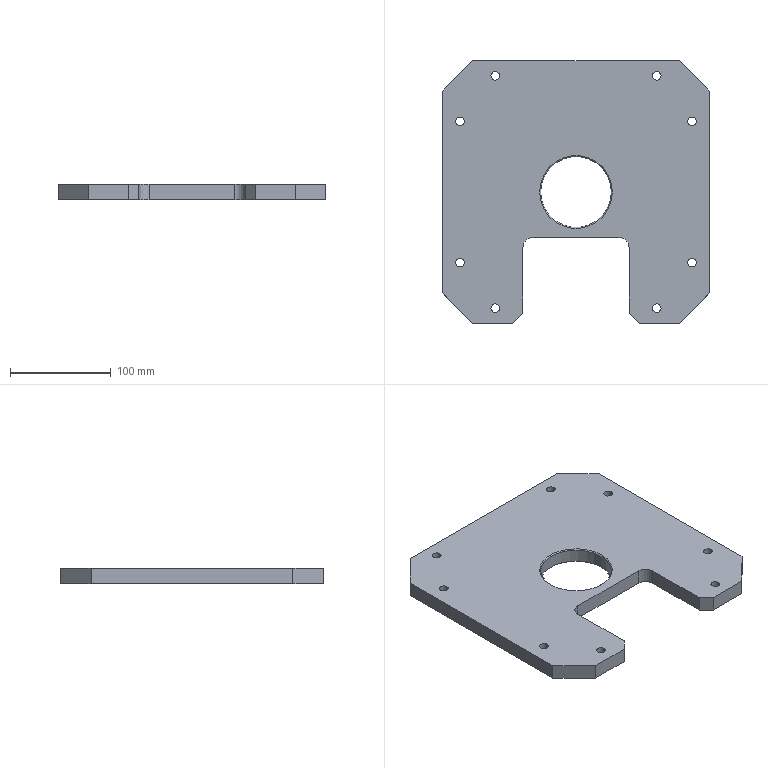Part | SolidWorks | features Chamfer 3, Cut 1, Extrusion 1, Fillet 1, HoleWzd 1, ICE 1 | 1 solid | 40 faces | box 265 x 260 x 15 mm | volume 807011 mm3 | cylinder 20 | plane 16 | cone 4 | commonest cylinder face diameters 8.5 x16 20 x2 70 x2
STEP:
#1=CARTESIAN_POINT('',(-35.,0.,14.));
#2=VERTEX_POINT('',#1);
#3=CARTESIAN_POINT('',(35.,0.,14.));
#4=VERTEX_POINT('',#3);
#5=CARTESIAN_POINT('',(0.,0.,14.));
#6=DIRECTION('',(0.,0.,1.));
#7=DIRECTION('',(-1.,0.,0.));
#8=AXIS2_PLACEMENT_3D('',#5,#6,#7);
#9=CIRCLE('',#8,35.);
#10=EDGE_CURVE('',#2,#4,#9,.T.);
#11=ORIENTED_EDGE('',*,*,#10,.F.);
#12=CARTESIAN_POINT('',(-36.,0.,15.));
#13=VERTEX_POINT('',#12);
#14=CARTESIAN_POINT('',(-36.,0.,15.));
#15=DIRECTION('',(-0.7071,0.,0.7071));
#16=VECTOR('',#15,1000.);
#17=LINE('',#14,#16);
#18=EDGE_CURVE('',#2,#13,#17,.T.);
#19=ORIENTED_EDGE('',*,*,#18,.T.);
#20=CARTESIAN_POINT('',(36.,0.,15.));
#21=VERTEX_POINT('',#20);
#22=CARTESIAN_POINT('',(0.,0.,15.));
#23=DIRECTION('',(0.,0.,-1.));
#24=DIRECTION('',(-1.,0.,0.));
#25=AXIS2_PLACEMENT_3D('',#22,#23,#24);
#26=CIRCLE('',#25,36.);
#27=EDGE_CURVE('',#21,#13,#26,.T.);
#28=ORIENTED_EDGE('',*,*,#27,.F.);
#29=CARTESIAN_POINT('',(36.,0.,15.));
#30=DIRECTION('',(0.7071,0.,0.7071));
#31=VECTOR('',#30,1000.);
#32=LINE('',#29,#31);
#33=EDGE_CURVE('',#4,#21,#32,.T.);
#34=ORIENTED_EDGE('',*,*,#33,.F.);
#35=EDGE_LOOP('',(#11,#19,#28,#34));
#36=FACE_OUTER_BOUND('',#35,.T.);
#37=CARTESIAN_POINT('',(0.,0.,15.));
#38=DIRECTION('',(0.,0.,1.));
#39=DIRECTION('',(1.,0.,0.));
#40=AXIS2_PLACEMENT_3D('',#37,#38,#39);
#41=CONICAL_SURFACE('',#40,36.,0.7854);
#42=ADVANCED_FACE('',(#36),#41,.F.);
#43=CARTESIAN_POINT('',(35.,0.,1.));
#44=VERTEX_POINT('',#43);
#45=CARTESIAN_POINT('',(-35.,0.,1.));
#46=VERTEX_POINT('',#45);
#47=CARTESIAN_POINT('',(0.,0.,1.));
#48=DIRECTION('',(0.,0.,-1.));
#49=DIRECTION('',(-1.,0.,0.));
#50=AXIS2_PLACEMENT_3D('',#47,#48,#49);
#51=CIRCLE('',#50,35.);
#52=EDGE_CURVE('',#44,#46,#51,.T.);
#53=ORIENTED_EDGE('',*,*,#52,.F.);
#54=CARTESIAN_POINT('',(36.,0.,0.));
#55=VERTEX_POINT('',#54);
#56=CARTESIAN_POINT('',(35.,0.,1.));
#57=DIRECTION('',(0.7071,0.,-0.7071));
#58=VECTOR('',#57,1000.);
#59=LINE('',#56,#58);
#60=EDGE_CURVE('',#44,#55,#59,.T.);
#61=ORIENTED_EDGE('',*,*,#60,.T.);
#62=CARTESIAN_POINT('',(-36.,0.,0.));
#63=VERTEX_POINT('',#62);
#64=CARTESIAN_POINT('',(0.,0.,0.));
#65=DIRECTION('',(0.,0.,1.));
#66=DIRECTION('',(-1.,0.,0.));
#67=AXIS2_PLACEMENT_3D('',#64,#65,#66);
#68=CIRCLE('',#67,36.);
#69=EDGE_CURVE('',#63,#55,#68,.T.);
#70=ORIENTED_EDGE('',*,*,#69,.F.);
#71=CARTESIAN_POINT('',(-35.,0.,1.));
#72=DIRECTION('',(-0.7071,0.,-0.7071));
#73=VECTOR('',#72,1000.);
#74=LINE('',#71,#73);
#75=EDGE_CURVE('',#46,#63,#74,.T.);
#76=ORIENTED_EDGE('',*,*,#75,.F.);
#77=EDGE_LOOP('',(#53,#61,#70,#76));
#78=FACE_OUTER_BOUND('',#77,.T.);
#79=CARTESIAN_POINT('',(0.,0.,1.));
#80=DIRECTION('',(0.,0.,-1.));
#81=DIRECTION('',(-1.,0.,0.));
#82=AXIS2_PLACEMENT_3D('',#79,#80,#81);
#83=CONICAL_SURFACE('',#82,35.,0.7854);
#84=ADVANCED_FACE('',(#78),#83,.F.);
#85=ORIENTED_EDGE('',*,*,#10,.T.);
#86=CARTESIAN_POINT('',(35.,0.,15.));
#87=DIRECTION('',(0.,0.,-1.));
#88=VECTOR('',#87,1000.);
#89=LINE('',#86,#88);
#90=EDGE_CURVE('',#4,#44,#89,.T.);
#91=ORIENTED_EDGE('',*,*,#90,.T.);
#92=ORIENTED_EDGE('',*,*,#52,.T.);
#93=CARTESIAN_POINT('',(-35.,0.,15.));
#94=DIRECTION('',(0.,0.,-1.));
#95=VECTOR('',#94,1000.);
#96=LINE('',#93,#95);
#97=EDGE_CURVE('',#2,#46,#96,.T.);
#98=ORIENTED_EDGE('',*,*,#97,.F.);
#99=EDGE_LOOP('',(#85,#91,#92,#98));
#100=FACE_OUTER_BOUND('',#99,.T.);
#101=CARTESIAN_POINT('',(0.,0.,15.));
#102=DIRECTION('',(0.,0.,-1.));
#103=DIRECTION('',(-1.,0.,0.));
#104=AXIS2_PLACEMENT_3D('',#101,#102,#103);
#105=CYLINDRICAL_SURFACE('',#104,35.);
#106=ADVANCED_FACE('',(#100),#105,.F.);
#107=CARTESIAN_POINT('',(84.25,115.,15.));
#108=VERTEX_POINT('',#107);
#109=CARTESIAN_POINT('',(75.75,115.,15.));
#110=VERTEX_POINT('',#109);
#111=CARTESIAN_POINT('',(80.,115.,15.));
#112=DIRECTION('',(0.,0.,-1.));
#113=DIRECTION('',(-1.,0.,0.));
#114=AXIS2_PLACEMENT_3D('',#111,#112,#113);
#115=CIRCLE('',#114,4.25);
#116=EDGE_CURVE('',#108,#110,#115,.T.);
#117=ORIENTED_EDGE('',*,*,#116,.F.);
#118=CARTESIAN_POINT('',(84.25,115.,0.));
#119=VERTEX_POINT('',#118);
#120=CARTESIAN_POINT('',(84.25,115.,0.));
#121=DIRECTION('',(0.,0.,-1.));
#122=VECTOR('',#121,1000.);
#123=LINE('',#120,#122);
#124=EDGE_CURVE('',#108,#119,#123,.T.);
#125=ORIENTED_EDGE('',*,*,#124,.T.);
#126=CARTESIAN_POINT('',(75.75,115.,0.));
#127=VERTEX_POINT('',#126);
#128=CARTESIAN_POINT('',(80.,115.,0.));
#129=DIRECTION('',(0.,0.,-1.));
#130=DIRECTION('',(-1.,0.,0.));
#131=AXIS2_PLACEMENT_3D('',#128,#129,#130);
#132=CIRCLE('',#131,4.25);
#133=EDGE_CURVE('',#119,#127,#132,.T.);
#134=ORIENTED_EDGE('',*,*,#133,.T.);
#135=CARTESIAN_POINT('',(75.75,115.,0.));
#136=DIRECTION('',(0.,0.,-1.));
#137=VECTOR('',#136,1000.);
#138=LINE('',#135,#137);
#139=EDGE_CURVE('',#110,#127,#138,.T.);
#140=ORIENTED_EDGE('',*,*,#139,.F.);
#141=EDGE_LOOP('',(#117,#125,#134,#140));
#142=FACE_OUTER_BOUND('',#141,.T.);
#143=CARTESIAN_POINT('',(80.,115.,0.));
#144=DIRECTION('',(0.,0.,-1.));
#145=DIRECTION('',(-1.,0.,0.));
#146=AXIS2_PLACEMENT_3D('',#143,#144,#145);
#147=CYLINDRICAL_SURFACE('',#146,4.25);
#148=ADVANCED_FACE('',(#142),#147,.F.);
#149=CARTESIAN_POINT('',(119.25,70.,15.));
#150=VERTEX_POINT('',#149);
#151=CARTESIAN_POINT('',(110.75,70.,15.));
#152=VERTEX_POINT('',#151);
#153=CARTESIAN_POINT('',(115.,70.,15.));
#154=DIRECTION('',(0.,0.,-1.));
#155=DIRECTION('',(-1.,0.,0.));
#156=AXIS2_PLACEMENT_3D('',#153,#154,#155);
#157=CIRCLE('',#156,4.25);
#158=EDGE_CURVE('',#150,#152,#157,.T.);
#159=ORIENTED_EDGE('',*,*,#158,.F.);
#160=CARTESIAN_POINT('',(119.25,70.,0.));
#161=VERTEX_POINT('',#160);
#162=CARTESIAN_POINT('',(119.25,70.,0.));
#163=DIRECTION('',(0.,0.,-1.));
#164=VECTOR('',#163,1000.);
#165=LINE('',#162,#164);
#166=EDGE_CURVE('',#150,#161,#165,.T.);
#167=ORIENTED_EDGE('',*,*,#166,.T.);
#168=CARTESIAN_POINT('',(110.75,70.,0.));
#169=VERTEX_POINT('',#168);
#170=CARTESIAN_POINT('',(115.,70.,0.));
#171=DIRECTION('',(0.,0.,-1.));
#172=DIRECTION('',(-1.,0.,0.));
#173=AXIS2_PLACEMENT_3D('',#170,#171,#172);
#174=CIRCLE('',#173,4.25);
#175=EDGE_CURVE('',#161,#169,#174,.T.);
#176=ORIENTED_EDGE('',*,*,#175,.T.);
#177=CARTESIAN_POINT('',(110.75,70.,0.));
#178=DIRECTION('',(0.,0.,-1.));
#179=VECTOR('',#178,1000.);
#180=LINE('',#177,#179);
#181=EDGE_CURVE('',#152,#169,#180,.T.);
#182=ORIENTED_EDGE('',*,*,#181,.F.);
#183=EDGE_LOOP('',(#159,#167,#176,#182));
#184=FACE_OUTER_BOUND('',#183,.T.);
#185=CARTESIAN_POINT('',(115.,70.,0.));
#186=DIRECTION('',(0.,0.,-1.));
#187=DIRECTION('',(-1.,0.,0.));
#188=AXIS2_PLACEMENT_3D('',#185,#186,#187);
#189=CYLINDRICAL_SURFACE('',#188,4.25);
#190=ADVANCED_FACE('',(#184),#189,.F.);
#191=CARTESIAN_POINT('',(119.25,-70.,15.));
#192=VERTEX_POINT('',#191);
#193=CARTESIAN_POINT('',(110.75,-70.,15.));
#194=VERTEX_POINT('',#193);
#195=CARTESIAN_POINT('',(115.,-70.,15.));
#196=DIRECTION('',(0.,0.,-1.));
#197=DIRECTION('',(-1.,0.,0.));
#198=AXIS2_PLACEMENT_3D('',#195,#196,#197);
#199=CIRCLE('',#198,4.25);
#200=EDGE_CURVE('',#192,#194,#199,.T.);
#201=ORIENTED_EDGE('',*,*,#200,.F.);
#202=CARTESIAN_POINT('',(119.25,-70.,0.));
#203=VERTEX_POINT('',#202);
#204=CARTESIAN_POINT('',(119.25,-70.,0.));
#205=DIRECTION('',(0.,0.,-1.));
#206=VECTOR('',#205,1000.);
#207=LINE('',#204,#206);
#208=EDGE_CURVE('',#192,#203,#207,.T.);
#209=ORIENTED_EDGE('',*,*,#208,.T.);
#210=CARTESIAN_POINT('',(110.75,-70.,0.));
#211=VERTEX_POINT('',#210);
#212=CARTESIAN_POINT('',(115.,-70.,0.));
#213=DIRECTION('',(0.,0.,-1.));
#214=DIRECTION('',(-1.,0.,0.));
#215=AXIS2_PLACEMENT_3D('',#212,#213,#214);
#216=CIRCLE('',#215,4.25);
#217=EDGE_CURVE('',#203,#211,#216,.T.);
#218=ORIENTED_EDGE('',*,*,#217,.T.);
#219=CARTESIAN_POINT('',(110.75,-70.,0.));
#220=DIRECTION('',(0.,0.,-1.));
#221=VECTOR('',#220,1000.);
#222=LINE('',#219,#221);
#223=EDGE_CURVE('',#194,#211,#222,.T.);
#224=ORIENTED_EDGE('',*,*,#223,.F.);
#225=EDGE_LOOP('',(#201,#209,#218,#224));
#226=FACE_OUTER_BOUND('',#225,.T.);
#227=CARTESIAN_POINT('',(115.,-70.,0.));
#228=DIRECTION('',(0.,0.,-1.));
#229=DIRECTION('',(-1.,0.,0.));
#230=AXIS2_PLACEMENT_3D('',#227,#228,#229);
#231=CYLINDRICAL_SURFACE('',#230,4.25);
#232=ADVANCED_FACE('',(#226),#231,.F.);
#233=CARTESIAN_POINT('',(84.25,-115.,15.));
#234=VERTEX_POINT('',#233);
#235=CARTESIAN_POINT('',(75.75,-115.,15.));
#236=VERTEX_POINT('',#235);
#237=CARTESIAN_POINT('',(80.,-115.,15.));
#238=DIRECTION('',(0.,0.,-1.));
#239=DIRECTION('',(-1.,0.,0.));
#240=AXIS2_PLACEMENT_3D('',#237,#238,#239);
#241=CIRCLE('',#240,4.25);
#242=EDGE_CURVE('',#234,#236,#241,.T.);
#243=ORIENTED_EDGE('',*,*,#242,.F.);
#244=CARTESIAN_POINT('',(84.25,-115.,0.));
#245=VERTEX_POINT('',#244);
#246=CARTESIAN_POINT('',(84.25,-115.,0.));
#247=DIRECTION('',(0.,0.,-1.));
#248=VECTOR('',#247,1000.);
#249=LINE('',#246,#248);
#250=EDGE_CURVE('',#234,#245,#249,.T.);
#251=ORIENTED_EDGE('',*,*,#250,.T.);
#252=CARTESIAN_POINT('',(75.75,-115.,0.));
#253=VERTEX_POINT('',#252);
#254=CARTESIAN_POINT('',(80.,-115.,0.));
#255=DIRECTION('',(0.,0.,-1.));
#256=DIRECTION('',(-1.,0.,0.));
#257=AXIS2_PLACEMENT_3D('',#254,#255,#256);
#258=CIRCLE('',#257,4.25);
#259=EDGE_CURVE('',#245,#253,#258,.T.);
#260=ORIENTED_EDGE('',*,*,#259,.T.);
#261=CARTESIAN_POINT('',(75.75,-115.,0.));
#262=DIRECTION('',(0.,0.,-1.));
#263=VECTOR('',#262,1000.);
#264=LINE('',#261,#263);
#265=EDGE_CURVE('',#236,#253,#264,.T.);
#266=ORIENTED_EDGE('',*,*,#265,.F.);
#267=EDGE_LOOP('',(#243,#251,#260,#266));
#268=FACE_OUTER_BOUND('',#267,.T.);
#269=CARTESIAN_POINT('',(80.,-115.,0.));
#270=DIRECTION('',(0.,0.,-1.));
#271=DIRECTION('',(-1.,0.,0.));
#272=AXIS2_PLACEMENT_3D('',#269,#270,#271);
#273=CYLINDRICAL_SURFACE('',#272,4.25);
#274=ADVANCED_FACE('',(#268),#273,.F.);
#275=CARTESIAN_POINT('',(-75.75,-115.,15.));
#276=VERTEX_POINT('',#275);
#277=CARTESIAN_POINT('',(-84.25,-115.,15.));
#278=VERTEX_POINT('',#277);
#279=CARTESIAN_POINT('',(-80.,-115.,15.));
#280=DIRECTION('',(0.,0.,-1.));
#281=DIRECTION('',(-1.,0.,0.));
#282=AXIS2_PLACEMENT_3D('',#279,#280,#281);
#283=CIRCLE('',#282,4.25);
#284=EDGE_CURVE('',#276,#278,#283,.T.);
#285=ORIENTED_EDGE('',*,*,#284,.F.);
#286=CARTESIAN_POINT('',(-75.75,-115.,0.));
#287=VERTEX_POINT('',#286);
#288=CARTESIAN_POINT('',(-75.75,-115.,0.));
#289=DIRECTION('',(0.,0.,-1.));
#290=VECTOR('',#289,1000.);
#291=LINE('',#288,#290);
#292=EDGE_CURVE('',#276,#287,#291,.T.);
#293=ORIENTED_EDGE('',*,*,#292,.T.);
#294=CARTESIAN_POINT('',(-84.25,-115.,0.));
#295=VERTEX_POINT('',#294);
#296=CARTESIAN_POINT('',(-80.,-115.,0.));
#297=DIRECTION('',(0.,0.,-1.));
#298=DIRECTION('',(-1.,0.,0.));
#299=AXIS2_PLACEMENT_3D('',#296,#297,#298);
#300=CIRCLE('',#299,4.25);
#301=EDGE_CURVE('',#287,#295,#300,.T.);
#302=ORIENTED_EDGE('',*,*,#301,.T.);
#303=CARTESIAN_POINT('',(-84.25,-115.,0.));
#304=DIRECTION('',(0.,0.,-1.));
#305=VECTOR('',#304,1000.);
#306=LINE('',#303,#305);
#307=EDGE_CURVE('',#278,#295,#306,.T.);
#308=ORIENTED_EDGE('',*,*,#307,.F.);
#309=EDGE_LOOP('',(#285,#293,#302,#308));
#310=FACE_OUTER_BOUND('',#309,.T.);
#311=CARTESIAN_POINT('',(-80.,-115.,0.));
#312=DIRECTION('',(0.,0.,-1.));
#313=DIRECTION('',(-1.,0.,0.));
#314=AXIS2_PLACEMENT_3D('',#311,#312,#313);
#315=CYLINDRICAL_SURFACE('',#314,4.25);
#316=ADVANCED_FACE('',(#310),#315,.F.);
#317=CARTESIAN_POINT('',(-110.75,-70.,15.));
#318=VERTEX_POINT('',#317);
#319=CARTESIAN_POINT('',(-119.25,-70.,15.));
#320=VERTEX_POINT('',#319);
#321=CARTESIAN_POINT('',(-115.,-70.,15.));
#322=DIRECTION('',(0.,0.,-1.));
#323=DIRECTION('',(-1.,0.,0.));
#324=AXIS2_PLACEMENT_3D('',#321,#322,#323);
#325=CIRCLE('',#324,4.25);
#326=EDGE_CURVE('',#318,#320,#325,.T.);
#327=ORIENTED_EDGE('',*,*,#326,.F.);
#328=CARTESIAN_POINT('',(-110.75,-70.,0.));
#329=VERTEX_POINT('',#328);
#330=CARTESIAN_POINT('',(-110.75,-70.,0.));
#331=DIRECTION('',(0.,0.,-1.));
#332=VECTOR('',#331,1000.);
#333=LINE('',#330,#332);
#334=EDGE_CURVE('',#318,#329,#333,.T.);
#335=ORIENTED_EDGE('',*,*,#334,.T.);
#336=CARTESIAN_POINT('',(-119.25,-70.,0.));
#337=VERTEX_POINT('',#336);
#338=CARTESIAN_POINT('',(-115.,-70.,0.));
#339=DIRECTION('',(0.,0.,-1.));
#340=DIRECTION('',(-1.,0.,0.));
#341=AXIS2_PLACEMENT_3D('',#338,#339,#340);
#342=CIRCLE('',#341,4.25);
#343=EDGE_CURVE('',#329,#337,#342,.T.);
#344=ORIENTED_EDGE('',*,*,#343,.T.);
#345=CARTESIAN_POINT('',(-119.25,-70.,0.));
#346=DIRECTION('',(0.,0.,-1.));
#347=VECTOR('',#346,1000.);
#348=LINE('',#345,#347);
#349=EDGE_CURVE('',#320,#337,#348,.T.);
#350=ORIENTED_EDGE('',*,*,#349,.F.);
#351=EDGE_LOOP('',(#327,#335,#344,#350));
#352=FACE_OUTER_BOUND('',#351,.T.);
#353=CARTESIAN_POINT('',(-115.,-70.,0.));
#354=DIRECTION('',(0.,0.,-1.));
#355=DIRECTION('',(-1.,0.,0.));
#356=AXIS2_PLACEMENT_3D('',#353,#354,#355);
#357=CYLINDRICAL_SURFACE('',#356,4.25);
#358=ADVANCED_FACE('',(#352),#357,.F.);
#359=CARTESIAN_POINT('',(-110.75,70.,15.));
#360=VERTEX_POINT('',#359);
#361=CARTESIAN_POINT('',(-119.25,70.,15.));
#362=VERTEX_POINT('',#361);
#363=CARTESIAN_POINT('',(-115.,70.,15.));
#364=DIRECTION('',(0.,0.,-1.));
#365=DIRECTION('',(-1.,0.,0.));
#366=AXIS2_PLACEMENT_3D('',#363,#364,#365);
#367=CIRCLE('',#366,4.25);
#368=EDGE_CURVE('',#360,#362,#367,.T.);
#369=ORIENTED_EDGE('',*,*,#368,.F.);
#370=CARTESIAN_POINT('',(-110.75,70.,0.));
#371=VERTEX_POINT('',#370);
#372=CARTESIAN_POINT('',(-110.75,70.,0.));
#373=DIRECTION('',(0.,0.,-1.));
#374=VECTOR('',#373,1000.);
#375=LINE('',#372,#374);
#376=EDGE_CURVE('',#360,#371,#375,.T.);
#377=ORIENTED_EDGE('',*,*,#376,.T.);
#378=CARTESIAN_POINT('',(-119.25,70.,0.));
#379=VERTEX_POINT('',#378);
#380=CARTESIAN_POINT('',(-115.,70.,0.));
#381=DIRECTION('',(0.,0.,-1.));
#382=DIRECTION('',(-1.,0.,0.));
#383=AXIS2_PLACEMENT_3D('',#380,#381,#382);
#384=CIRCLE('',#383,4.25);
#385=EDGE_CURVE('',#371,#379,#384,.T.);
#386=ORIENTED_EDGE('',*,*,#385,.T.);
#387=CARTESIAN_POINT('',(-119.25,70.,0.));
#388=DIRECTION('',(0.,0.,-1.));
#389=VECTOR('',#388,1000.);
#390=LINE('',#387,#389);
#391=EDGE_CURVE('',#362,#379,#390,.T.);
#392=ORIENTED_EDGE('',*,*,#391,.F.);
#393=EDGE_LOOP('',(#369,#377,#386,#392));
#394=FACE_OUTER_BOUND('',#393,.T.);
#395=CARTESIAN_POINT('',(-115.,70.,0.));
#396=DIRECTION('',(0.,0.,-1.));
#397=DIRECTION('',(-1.,0.,0.));
#398=AXIS2_PLACEMENT_3D('',#395,#396,#397);
#399=CYLINDRICAL_SURFACE('',#398,4.25);
#400=ADVANCED_FACE('',(#394),#399,.F.);
#401=CARTESIAN_POINT('',(-75.75,115.,15.));
#402=VERTEX_POINT('',#401);
#403=CARTESIAN_POINT('',(-84.25,115.,15.));
#404=VERTEX_POINT('',#403);
#405=CARTESIAN_POINT('',(-80.,115.,15.));
#406=DIRECTION('',(0.,0.,-1.));
#407=DIRECTION('',(-1.,0.,0.));
#408=AXIS2_PLACEMENT_3D('',#405,#406,#407);
#409=CIRCLE('',#408,4.25);
#410=EDGE_CURVE('',#402,#404,#409,.T.);
#411=ORIENTED_EDGE('',*,*,#410,.F.);
#412=CARTESIAN_POINT('',(-75.75,115.,0.));
#413=VERTEX_POINT('',#412);
#414=CARTESIAN_POINT('',(-75.75,115.,0.));
#415=DIRECTION('',(0.,0.,-1.));
#416=VECTOR('',#415,1000.);
#417=LINE('',#414,#416);
#418=EDGE_CURVE('',#402,#413,#417,.T.);
#419=ORIENTED_EDGE('',*,*,#418,.T.);
#420=CARTESIAN_POINT('',(-84.25,115.,0.));
#421=VERTEX_POINT('',#420);
#422=CARTESIAN_POINT('',(-80.,115.,0.));
#423=DIRECTION('',(0.,0.,-1.));
#424=DIRECTION('',(-1.,0.,0.));
#425=AXIS2_PLACEMENT_3D('',#422,#423,#424);
#426=CIRCLE('',#425,4.25);
#427=EDGE_CURVE('',#413,#421,#426,.T.);
#428=ORIENTED_EDGE('',*,*,#427,.T.);
#429=CARTESIAN_POINT('',(-84.25,115.,0.));
#430=DIRECTION('',(0.,0.,-1.));
#431=VECTOR('',#430,1000.);
#432=LINE('',#429,#431);
#433=EDGE_CURVE('',#404,#421,#432,.T.);
#434=ORIENTED_EDGE('',*,*,#433,.F.);
#435=EDGE_LOOP('',(#411,#419,#428,#434));
#436=FACE_OUTER_BOUND('',#435,.T.);
#437=CARTESIAN_POINT('',(-80.,115.,0.));
#438=DIRECTION('',(0.,0.,-1.));
#439=DIRECTION('',(-1.,0.,0.));
#440=AXIS2_PLACEMENT_3D('',#437,#438,#439);
#441=CYLINDRICAL_SURFACE('',#440,4.25);
#442=ADVANCED_FACE('',(#436),#441,.F.);
#443=CARTESIAN_POINT('',(62.5,-130.,15.));
#444=VERTEX_POINT('',#443);
#445=CARTESIAN_POINT('',(102.5,-130.,15.));
#446=VERTEX_POINT('',#445);
#447=CARTESIAN_POINT('',(-132.5,-130.,15.));
#448=DIRECTION('',(1.,0.,0.));
#449=VECTOR('',#448,1000.);
#450=LINE('',#447,#449);
#451=EDGE_CURVE('',#444,#446,#450,.T.);
#452=ORIENTED_EDGE('',*,*,#451,.F.);
#453=CARTESIAN_POINT('',(62.5,-130.,0.));
#454=VERTEX_POINT('',#453);
#455=CARTESIAN_POINT('',(62.5,-130.,15.));
#456=DIRECTION('',(0.,0.,-1.));
#457=VECTOR('',#456,1000.);
#458=LINE('',#455,#457);
#459=EDGE_CURVE('',#444,#454,#458,.T.);
#460=ORIENTED_EDGE('',*,*,#459,.T.);
#461=CARTESIAN_POINT('',(102.5,-130.,0.));
#462=VERTEX_POINT('',#461);
#463=CARTESIAN_POINT('',(-132.5,-130.,0.));
#464=DIRECTION('',(1.,0.,0.));
#465=VECTOR('',#464,1000.);
#466=LINE('',#463,#465);
#467=EDGE_CURVE('',#454,#462,#466,.T.);
#468=ORIENTED_EDGE('',*,*,#467,.T.);
#469=CARTESIAN_POINT('',(102.5,-130.,15.));
#470=DIRECTION('',(0.,0.,1.));
#471=VECTOR('',#470,1000.);
#472=LINE('',#469,#471);
#473=EDGE_CURVE('',#462,#446,#472,.T.);
#474=ORIENTED_EDGE('',*,*,#473,.T.);
#475=EDGE_LOOP('',(#452,#460,#468,#474));
#476=FACE_OUTER_BOUND('',#475,.T.);
#477=CARTESIAN_POINT('',(-132.5,-130.,15.));
#478=DIRECTION('',(0.,1.,0.));
#479=DIRECTION('',(0.,0.,1.));
#480=AXIS2_PLACEMENT_3D('',#477,#478,#479);
#481=PLANE('',#480);
#482=ADVANCED_FACE('',(#476),#481,.F.);
#483=CARTESIAN_POINT('',(132.5,-100.,15.));
#484=VERTEX_POINT('',#483);
#485=CARTESIAN_POINT('',(132.5,100.,15.));
#486=VERTEX_POINT('',#485);
#487=CARTESIAN_POINT('',(132.5,-130.,15.));
#488=DIRECTION('',(0.,1.,0.));
#489=VECTOR('',#488,1000.);
#490=LINE('',#487,#489);
#491=EDGE_CURVE('',#484,#486,#490,.T.);
#492=ORIENTED_EDGE('',*,*,#491,.F.);
#493=CARTESIAN_POINT('',(132.5,-100.,0.));
#494=VERTEX_POINT('',#493);
#495=CARTESIAN_POINT('',(132.5,-100.,15.));
#496=DIRECTION('',(0.,0.,-1.));
#497=VECTOR('',#496,1000.);
#498=LINE('',#495,#497);
#499=EDGE_CURVE('',#484,#494,#498,.T.);
#500=ORIENTED_EDGE('',*,*,#499,.T.);
#501=CARTESIAN_POINT('',(132.5,100.,0.));
#502=VERTEX_POINT('',#501);
#503=CARTESIAN_POINT('',(132.5,-130.,0.));
#504=DIRECTION('',(0.,1.,0.));
#505=VECTOR('',#504,1000.);
#506=LINE('',#503,#505);
#507=EDGE_CURVE('',#494,#502,#506,.T.);
#508=ORIENTED_EDGE('',*,*,#507,.T.);
#509=CARTESIAN_POINT('',(132.5,100.,15.));
#510=DIRECTION('',(0.,0.,1.));
#511=VECTOR('',#510,1000.);
#512=LINE('',#509,#511);
#513=EDGE_CURVE('',#502,#486,#512,.T.);
#514=ORIENTED_EDGE('',*,*,#513,.T.);
#515=EDGE_LOOP('',(#492,#500,#508,#514));
#516=FACE_OUTER_BOUND('',#515,.T.);
#517=CARTESIAN_POINT('',(132.5,-130.,15.));
#518=DIRECTION('',(-1.,0.,0.));
#519=DIRECTION('',(0.,0.,1.));
#520=AXIS2_PLACEMENT_3D('',#517,#518,#519);
#521=PLANE('',#520);
#522=ADVANCED_FACE('',(#516),#521,.F.);
#523=CARTESIAN_POINT('',(102.5,130.,0.));
#524=VERTEX_POINT('',#523);
#525=CARTESIAN_POINT('',(-102.5,130.,0.));
#526=VERTEX_POINT('',#525);
#527=CARTESIAN_POINT('',(-132.5,130.,0.));
#528=DIRECTION('',(-1.,0.,0.));
#529=VECTOR('',#528,1000.);
#530=LINE('',#527,#529);
#531=EDGE_CURVE('',#524,#526,#530,.T.);
#532=ORIENTED_EDGE('',*,*,#531,.T.);
#533=CARTESIAN_POINT('',(-102.5,130.,15.));
#534=VERTEX_POINT('',#533);
#535=CARTESIAN_POINT('',(-102.5,130.,15.));
#536=DIRECTION('',(0.,0.,1.));
#537=VECTOR('',#536,1000.);
#538=LINE('',#535,#537);
#539=EDGE_CURVE('',#526,#534,#538,.T.);
#540=ORIENTED_EDGE('',*,*,#539,.T.);
#541=CARTESIAN_POINT('',(102.5,130.,15.));
#542=VERTEX_POINT('',#541);
#543=CARTESIAN_POINT('',(-132.5,130.,15.));
#544=DIRECTION('',(-1.,0.,0.));
#545=VECTOR('',#544,1000.);
#546=LINE('',#543,#545);
#547=EDGE_CURVE('',#542,#534,#546,.T.);
#548=ORIENTED_EDGE('',*,*,#547,.F.);
#549=CARTESIAN_POINT('',(102.5,130.,15.));
#550=DIRECTION('',(0.,0.,-1.));
#551=VECTOR('',#550,1000.);
#552=LINE('',#549,#551);
#553=EDGE_CURVE('',#542,#524,#552,.T.);
#554=ORIENTED_EDGE('',*,*,#553,.T.);
#555=EDGE_LOOP('',(#532,#540,#548,#554));
#556=FACE_OUTER_BOUND('',#555,.T.);
#557=CARTESIAN_POINT('',(-132.5,130.,15.));
#558=DIRECTION('',(0.,-1.,0.));
#559=DIRECTION('',(0.,0.,-1.));
#560=AXIS2_PLACEMENT_3D('',#557,#558,#559);
#561=PLANE('',#560);
#562=ADVANCED_FACE('',(#556),#561,.F.);
#563=CARTESIAN_POINT('',(-132.5,100.,0.));
#564=VERTEX_POINT('',#563);
#565=CARTESIAN_POINT('',(-132.5,-100.,0.));
#566=VERTEX_POINT('',#565);
#567=CARTESIAN_POINT('',(-132.5,-130.,0.));
#568=DIRECTION('',(0.,-1.,0.));
#569=VECTOR('',#568,1000.);
#570=LINE('',#567,#569);
#571=EDGE_CURVE('',#564,#566,#570,.T.);
#572=ORIENTED_EDGE('',*,*,#571,.T.);
#573=CARTESIAN_POINT('',(-132.5,-100.,15.));
#574=VERTEX_POINT('',#573);
#575=CARTESIAN_POINT('',(-132.5,-100.,15.));
#576=DIRECTION('',(0.,0.,1.));
#577=VECTOR('',#576,1000.);
#578=LINE('',#575,#577);
#579=EDGE_CURVE('',#566,#574,#578,.T.);
#580=ORIENTED_EDGE('',*,*,#579,.T.);
#581=CARTESIAN_POINT('',(-132.5,100.,15.));
#582=VERTEX_POINT('',#581);
#583=CARTESIAN_POINT('',(-132.5,-130.,15.));
#584=DIRECTION('',(0.,-1.,0.));
#585=VECTOR('',#584,1000.);
#586=LINE('',#583,#585);
#587=EDGE_CURVE('',#582,#574,#586,.T.);
#588=ORIENTED_EDGE('',*,*,#587,.F.);
#589=CARTESIAN_POINT('',(-132.5,100.,15.));
#590=DIRECTION('',(0.,0.,-1.));
#591=VECTOR('',#590,1000.);
#592=LINE('',#589,#591);
#593=EDGE_CURVE('',#582,#564,#592,.T.);
#594=ORIENTED_EDGE('',*,*,#593,.T.);
#595=EDGE_LOOP('',(#572,#580,#588,#594));
#596=FACE_OUTER_BOUND('',#595,.T.);
#597=CARTESIAN_POINT('',(-132.5,-130.,15.));
#598=DIRECTION('',(1.,0.,0.));
#599=DIRECTION('',(0.,0.,-1.));
#600=AXIS2_PLACEMENT_3D('',#597,#598,#599);
#601=PLANE('',#600);
#602=ADVANCED_FACE('',(#596),#601,.F.);
#603=CARTESIAN_POINT('',(-102.5,-130.,0.));
#604=VERTEX_POINT('',#603);
#605=CARTESIAN_POINT('',(-62.5,-130.,0.));
#606=VERTEX_POINT('',#605);
#607=CARTESIAN_POINT('',(-132.5,-130.,0.));
#608=DIRECTION('',(1.,0.,0.));
#609=VECTOR('',#608,1000.);
#610=LINE('',#607,#609);
#611=EDGE_CURVE('',#604,#606,#610,.T.);
#612=ORIENTED_EDGE('',*,*,#611,.T.);
#613=CARTESIAN_POINT('',(-62.5,-130.,15.));
#614=VERTEX_POINT('',#613);
#615=CARTESIAN_POINT('',(-62.5,-130.,15.));
#616=DIRECTION('',(0.,0.,1.));
#617=VECTOR('',#616,1000.);
#618=LINE('',#615,#617);
#619=EDGE_CURVE('',#606,#614,#618,.T.);
#620=ORIENTED_EDGE('',*,*,#619,.T.);
#621=CARTESIAN_POINT('',(-102.5,-130.,15.));
#622=VERTEX_POINT('',#621);
#623=CARTESIAN_POINT('',(-132.5,-130.,15.));
#624=DIRECTION('',(1.,0.,0.));
#625=VECTOR('',#624,1000.);
#626=LINE('',#623,#625);
#627=EDGE_CURVE('',#622,#614,#626,.T.);
#628=ORIENTED_EDGE('',*,*,#627,.F.);
#629=CARTESIAN_POINT('',(-102.5,-130.,15.));
#630=DIRECTION('',(0.,0.,-1.));
#631=VECTOR('',#630,1000.);
#632=LINE('',#629,#631);
#633=EDGE_CURVE('',#622,#604,#632,.T.);
#634=ORIENTED_EDGE('',*,*,#633,.T.);
#635=EDGE_LOOP('',(#612,#620,#628,#634));
#636=FACE_OUTER_BOUND('',#635,.T.);
#637=CARTESIAN_POINT('',(-132.5,-130.,15.));
#638=DIRECTION('',(0.,1.,0.));
#639=DIRECTION('',(0.,0.,1.));
#640=AXIS2_PLACEMENT_3D('',#637,#638,#639);
#641=PLANE('',#640);
#642=ADVANCED_FACE('',(#636),#641,.F.);
#643=ORIENTED_EDGE('',*,*,#27,.T.);
#644=CARTESIAN_POINT('',(0.,0.,15.));
#645=DIRECTION('',(0.,0.,-1.));
#646=DIRECTION('',(-1.,0.,0.));
#647=AXIS2_PLACEMENT_3D('',#644,#645,#646);
#648=CIRCLE('',#647,36.);
#649=EDGE_CURVE('',#13,#21,#648,.T.);
#650=ORIENTED_EDGE('',*,*,#649,.T.);
#651=EDGE_LOOP('',(#643,#650));
#652=FACE_BOUND('',#651,.T.);
#653=CARTESIAN_POINT('',(80.,115.,15.));
#654=DIRECTION('',(0.,0.,-1.));
#655=DIRECTION('',(-1.,0.,0.));
#656=AXIS2_PLACEMENT_3D('',#653,#654,#655);
#657=CIRCLE('',#656,4.25);
#658=EDGE_CURVE('',#110,#108,#657,.T.);
#659=ORIENTED_EDGE('',*,*,#658,.T.);
#660=ORIENTED_EDGE('',*,*,#116,.T.);
#661=EDGE_LOOP('',(#659,#660));
#662=FACE_BOUND('',#661,.T.);
#663=CARTESIAN_POINT('',(115.,70.,15.));
#664=DIRECTION('',(0.,0.,-1.));
#665=DIRECTION('',(-1.,0.,0.));
#666=AXIS2_PLACEMENT_3D('',#663,#664,#665);
#667=CIRCLE('',#666,4.25);
#668=EDGE_CURVE('',#152,#150,#667,.T.);
#669=ORIENTED_EDGE('',*,*,#668,.T.);
#670=ORIENTED_EDGE('',*,*,#158,.T.);
#671=EDGE_LOOP('',(#669,#670));
#672=FACE_BOUND('',#671,.T.);
#673=CARTESIAN_POINT('',(115.,-70.,15.));
#674=DIRECTION('',(0.,0.,-1.));
#675=DIRECTION('',(-1.,0.,0.));
#676=AXIS2_PLACEMENT_3D('',#673,#674,#675);
#677=CIRCLE('',#676,4.25);
#678=EDGE_CURVE('',#194,#192,#677,.T.);
#679=ORIENTED_EDGE('',*,*,#678,.T.);
#680=ORIENTED_EDGE('',*,*,#200,.T.);
#681=EDGE_LOOP('',(#679,#680));
#682=FACE_BOUND('',#681,.T.);
#683=CARTESIAN_POINT('',(80.,-115.,15.));
#684=DIRECTION('',(0.,0.,-1.));
#685=DIRECTION('',(-1.,0.,0.));
#686=AXIS2_PLACEMENT_3D('',#683,#684,#685);
#687=CIRCLE('',#686,4.25);
#688=EDGE_CURVE('',#236,#234,#687,.T.);
#689=ORIENTED_EDGE('',*,*,#688,.T.);
#690=ORIENTED_EDGE('',*,*,#242,.T.);
#691=EDGE_LOOP('',(#689,#690));
#692=FACE_BOUND('',#691,.T.);
#693=CARTESIAN_POINT('',(-80.,-115.,15.));
#694=DIRECTION('',(0.,0.,-1.));
#695=DIRECTION('',(-1.,0.,0.));
#696=AXIS2_PLACEMENT_3D('',#693,#694,#695);
#697=CIRCLE('',#696,4.25);
#698=EDGE_CURVE('',#278,#276,#697,.T.);
#699=ORIENTED_EDGE('',*,*,#698,.T.);
#700=ORIENTED_EDGE('',*,*,#284,.T.);
#701=EDGE_LOOP('',(#699,#700));
#702=FACE_BOUND('',#701,.T.);
#703=CARTESIAN_POINT('',(-115.,-70.,15.));
#704=DIRECTION('',(0.,0.,-1.));
#705=DIRECTION('',(-1.,0.,0.));
#706=AXIS2_PLACEMENT_3D('',#703,#704,#705);
#707=CIRCLE('',#706,4.25);
#708=EDGE_CURVE('',#320,#318,#707,.T.);
#709=ORIENTED_EDGE('',*,*,#708,.T.);
#710=ORIENTED_EDGE('',*,*,#326,.T.);
#711=EDGE_LOOP('',(#709,#710));
#712=FACE_BOUND('',#711,.T.);
#713=CARTESIAN_POINT('',(-115.,70.,15.));
#714=DIRECTION('',(0.,0.,-1.));
#715=DIRECTION('',(-1.,0.,0.));
#716=AXIS2_PLACEMENT_3D('',#713,#714,#715);
#717=CIRCLE('',#716,4.25);
#718=EDGE_CURVE('',#362,#360,#717,.T.);
#719=ORIENTED_EDGE('',*,*,#718,.T.);
#720=ORIENTED_EDGE('',*,*,#368,.T.);
#721=EDGE_LOOP('',(#719,#720));
#722=FACE_BOUND('',#721,.T.);
#723=CARTESIAN_POINT('',(-80.,115.,15.));
#724=DIRECTION('',(0.,0.,-1.));
#725=DIRECTION('',(-1.,0.,0.));
#726=AXIS2_PLACEMENT_3D('',#723,#724,#725);
#727=CIRCLE('',#726,4.25);
#728=EDGE_CURVE('',#404,#402,#727,.T.);
#729=ORIENTED_EDGE('',*,*,#728,.T.);
#730=ORIENTED_EDGE('',*,*,#410,.T.);
#731=EDGE_LOOP('',(#729,#730));
#732=FACE_BOUND('',#731,.T.);
#733=ORIENTED_EDGE('',*,*,#627,.T.);
#734=CARTESIAN_POINT('',(-52.5,-120.,15.));
#735=VERTEX_POINT('',#734);
#736=CARTESIAN_POINT('',(-52.5,-120.,15.));
#737=DIRECTION('',(0.7071,0.7071,0.));
#738=VECTOR('',#737,1000.);
#739=LINE('',#736,#738);
#740=EDGE_CURVE('',#614,#735,#739,.T.);
#741=ORIENTED_EDGE('',*,*,#740,.T.);
#742=CARTESIAN_POINT('',(-52.5,-55.,15.));
#743=VERTEX_POINT('',#742);
#744=CARTESIAN_POINT('',(-52.5,-130.,15.));
#745=DIRECTION('',(0.,1.,0.));
#746=VECTOR('',#745,1000.);
#747=LINE('',#744,#746);
#748=EDGE_CURVE('',#735,#743,#747,.T.);
#749=ORIENTED_EDGE('',*,*,#748,.T.);
#750=CARTESIAN_POINT('',(-42.5,-45.,15.));
#751=VERTEX_POINT('',#750);
#752=CARTESIAN_POINT('',(-42.5,-55.,15.));
#753=DIRECTION('',(0.,0.,-1.));
#754=DIRECTION('',(-1.,0.,0.));
#755=AXIS2_PLACEMENT_3D('',#752,#753,#754);
#756=CIRCLE('',#755,10.);
#757=EDGE_CURVE('',#743,#751,#756,.T.);
#758=ORIENTED_EDGE('',*,*,#757,.T.);
#759=CARTESIAN_POINT('',(42.5,-45.,15.));
#760=VERTEX_POINT('',#759);
#761=CARTESIAN_POINT('',(52.5,-45.,15.));
#762=DIRECTION('',(1.,0.,0.));
#763=VECTOR('',#762,1000.);
#764=LINE('',#761,#763);
#765=EDGE_CURVE('',#751,#760,#764,.T.);
#766=ORIENTED_EDGE('',*,*,#765,.T.);
#767=CARTESIAN_POINT('',(52.5,-55.,15.));
#768=VERTEX_POINT('',#767);
#769=CARTESIAN_POINT('',(42.5,-55.,15.));
#770=DIRECTION('',(0.,0.,-1.));
#771=DIRECTION('',(-1.,0.,0.));
#772=AXIS2_PLACEMENT_3D('',#769,#770,#771);
#773=CIRCLE('',#772,10.);
#774=EDGE_CURVE('',#760,#768,#773,.T.);
#775=ORIENTED_EDGE('',*,*,#774,.T.);
#776=CARTESIAN_POINT('',(52.5,-120.,15.));
#777=VERTEX_POINT('',#776);
#778=CARTESIAN_POINT('',(52.5,-130.,15.));
#779=DIRECTION('',(0.,-1.,0.));
#780=VECTOR('',#779,1000.);
#781=LINE('',#778,#780);
#782=EDGE_CURVE('',#768,#777,#781,.T.);
#783=ORIENTED_EDGE('',*,*,#782,.T.);
#784=CARTESIAN_POINT('',(62.5,-130.,15.));
#785=DIRECTION('',(0.7071,-0.7071,0.));
#786=VECTOR('',#785,1000.);
#787=LINE('',#784,#786);
#788=EDGE_CURVE('',#777,#444,#787,.T.);
#789=ORIENTED_EDGE('',*,*,#788,.T.);
#790=ORIENTED_EDGE('',*,*,#451,.T.);
#791=CARTESIAN_POINT('',(132.5,-100.,15.));
#792=DIRECTION('',(0.7071,0.7071,0.));
#793=VECTOR('',#792,1000.);
#794=LINE('',#791,#793);
#795=EDGE_CURVE('',#446,#484,#794,.T.);
#796=ORIENTED_EDGE('',*,*,#795,.T.);
#797=ORIENTED_EDGE('',*,*,#491,.T.);
#798=CARTESIAN_POINT('',(102.5,130.,15.));
#799=DIRECTION('',(-0.7071,0.7071,0.));
#800=VECTOR('',#799,1000.);
#801=LINE('',#798,#800);
#802=EDGE_CURVE('',#486,#542,#801,.T.);
#803=ORIENTED_EDGE('',*,*,#802,.T.);
#804=ORIENTED_EDGE('',*,*,#547,.T.);
#805=CARTESIAN_POINT('',(-132.5,100.,15.));
#806=DIRECTION('',(-0.7071,-0.7071,0.));
#807=VECTOR('',#806,1000.);
#808=LINE('',#805,#807);
#809=EDGE_CURVE('',#534,#582,#808,.T.);
#810=ORIENTED_EDGE('',*,*,#809,.T.);
#811=ORIENTED_EDGE('',*,*,#587,.T.);
#812=CARTESIAN_POINT('',(-102.5,-130.,15.));
#813=DIRECTION('',(0.7071,-0.7071,0.));
#814=VECTOR('',#813,1000.);
#815=LINE('',#812,#814);
#816=EDGE_CURVE('',#574,#622,#815,.T.);
#817=ORIENTED_EDGE('',*,*,#816,.T.);
#818=EDGE_LOOP('',(#733,#741,#749,#758,#766,#775,#783,#789,#790,#796,#797,#803,#804,#810,#811,#817));
#819=FACE_OUTER_BOUND('',#818,.T.);
#820=CARTESIAN_POINT('',(0.,0.,15.));
#821=DIRECTION('',(0.,0.,-1.));
#822=DIRECTION('',(-1.,0.,0.));
#823=AXIS2_PLACEMENT_3D('',#820,#821,#822);
#824=PLANE('',#823);
#825=ADVANCED_FACE('',(#652,#662,#672,#682,#692,#702,#712,#722,#732,#819),#824,.F.);
#826=ORIENTED_EDGE('',*,*,#69,.T.);
#827=CARTESIAN_POINT('',(0.,0.,0.));
#828=DIRECTION('',(0.,0.,1.));
#829=DIRECTION('',(-1.,0.,0.));
#830=AXIS2_PLACEMENT_3D('',#827,#828,#829);
#831=CIRCLE('',#830,36.);
#832=EDGE_CURVE('',#55,#63,#831,.T.);
#833=ORIENTED_EDGE('',*,*,#832,.T.);
#834=EDGE_LOOP('',(#826,#833));
#835=FACE_BOUND('',#834,.T.);
#836=CARTESIAN_POINT('',(-52.5,-120.,0.));
#837=VERTEX_POINT('',#836);
#838=CARTESIAN_POINT('',(-52.5,-55.,0.));
#839=VERTEX_POINT('',#838);
#840=CARTESIAN_POINT('',(-52.5,-130.,0.));
#841=DIRECTION('',(0.,1.,0.));
#842=VECTOR('',#841,1000.);
#843=LINE('',#840,#842);
#844=EDGE_CURVE('',#837,#839,#843,.T.);
#845=ORIENTED_EDGE('',*,*,#844,.F.);
#846=CARTESIAN_POINT('',(33.75,-33.75,0.));
#847=DIRECTION('',(-0.7071,-0.7071,0.));
#848=VECTOR('',#847,1000.);
#849=LINE('',#846,#848);
#850=EDGE_CURVE('',#837,#606,#849,.T.);
#851=ORIENTED_EDGE('',*,*,#850,.T.);
#852=ORIENTED_EDGE('',*,*,#611,.F.);
#853=CARTESIAN_POINT('',(-116.25,-116.25,0.));
#854=DIRECTION('',(-0.7071,0.7071,0.));
#855=VECTOR('',#854,1000.);
#856=LINE('',#853,#855);
#857=EDGE_CURVE('',#604,#566,#856,.T.);
#858=ORIENTED_EDGE('',*,*,#857,.T.);
#859=ORIENTED_EDGE('',*,*,#571,.F.);
#860=CARTESIAN_POINT('',(-116.25,116.25,0.));
#861=DIRECTION('',(0.7071,0.7071,0.));
#862=VECTOR('',#861,1000.);
#863=LINE('',#860,#862);
#864=EDGE_CURVE('',#564,#526,#863,.T.);
#865=ORIENTED_EDGE('',*,*,#864,.T.);
#866=ORIENTED_EDGE('',*,*,#531,.F.);
#867=CARTESIAN_POINT('',(116.25,116.25,0.));
#868=DIRECTION('',(0.7071,-0.7071,0.));
#869=VECTOR('',#868,1000.);
#870=LINE('',#867,#869);
#871=EDGE_CURVE('',#524,#502,#870,.T.);
#872=ORIENTED_EDGE('',*,*,#871,.T.);
#873=ORIENTED_EDGE('',*,*,#507,.F.);
#874=CARTESIAN_POINT('',(116.25,-116.25,0.));
#875=DIRECTION('',(-0.7071,-0.7071,0.));
#876=VECTOR('',#875,1000.);
#877=LINE('',#874,#876);
#878=EDGE_CURVE('',#494,#462,#877,.T.);
#879=ORIENTED_EDGE('',*,*,#878,.T.);
#880=ORIENTED_EDGE('',*,*,#467,.F.);
#881=CARTESIAN_POINT('',(52.5,-120.,0.));
#882=VERTEX_POINT('',#881);
#883=CARTESIAN_POINT('',(-33.75,-33.75,0.));
#884=DIRECTION('',(-0.7071,0.7071,0.));
#885=VECTOR('',#884,1000.);
#886=LINE('',#883,#885);
#887=EDGE_CURVE('',#454,#882,#886,.T.);
#888=ORIENTED_EDGE('',*,*,#887,.T.);
#889=CARTESIAN_POINT('',(52.5,-55.,0.));
#890=VERTEX_POINT('',#889);
#891=CARTESIAN_POINT('',(52.5,-130.,0.));
#892=DIRECTION('',(0.,-1.,0.));
#893=VECTOR('',#892,1000.);
#894=LINE('',#891,#893);
#895=EDGE_CURVE('',#890,#882,#894,.T.);
#896=ORIENTED_EDGE('',*,*,#895,.F.);
#897=CARTESIAN_POINT('',(42.5,-45.,0.));
#898=VERTEX_POINT('',#897);
#899=CARTESIAN_POINT('',(42.5,-55.,0.));
#900=DIRECTION('',(0.,0.,1.));
#901=DIRECTION('',(-1.,0.,0.));
#902=AXIS2_PLACEMENT_3D('',#899,#900,#901);
#903=CIRCLE('',#902,10.);
#904=EDGE_CURVE('',#890,#898,#903,.T.);
#905=ORIENTED_EDGE('',*,*,#904,.T.);
#906=CARTESIAN_POINT('',(-42.5,-45.,0.));
#907=VERTEX_POINT('',#906);
#908=CARTESIAN_POINT('',(52.5,-45.,0.));
#909=DIRECTION('',(1.,0.,0.));
#910=VECTOR('',#909,1000.);
#911=LINE('',#908,#910);
#912=EDGE_CURVE('',#907,#898,#911,.T.);
#913=ORIENTED_EDGE('',*,*,#912,.F.);
#914=CARTESIAN_POINT('',(-42.5,-55.,0.));
#915=DIRECTION('',(0.,0.,1.));
#916=DIRECTION('',(-1.,0.,0.));
#917=AXIS2_PLACEMENT_3D('',#914,#915,#916);
#918=CIRCLE('',#917,10.);
#919=EDGE_CURVE('',#907,#839,#918,.T.);
#920=ORIENTED_EDGE('',*,*,#919,.T.);
#921=EDGE_LOOP('',(#845,#851,#852,#858,#859,#865,#866,#872,#873,#879,#880,#888,#896,#905,#913,#920));
#922=FACE_OUTER_BOUND('',#921,.T.);
#923=CARTESIAN_POINT('',(80.,115.,0.));
#924=DIRECTION('',(0.,0.,-1.));
#925=DIRECTION('',(-1.,0.,0.));
#926=AXIS2_PLACEMENT_3D('',#923,#924,#925);
#927=CIRCLE('',#926,4.25);
#928=EDGE_CURVE('',#127,#119,#927,.T.);
#929=ORIENTED_EDGE('',*,*,#928,.F.);
#930=ORIENTED_EDGE('',*,*,#133,.F.);
#931=EDGE_LOOP('',(#929,#930));
#932=FACE_BOUND('',#931,.T.);
#933=CARTESIAN_POINT('',(115.,70.,0.));
#934=DIRECTION('',(0.,0.,-1.));
#935=DIRECTION('',(-1.,0.,0.));
#936=AXIS2_PLACEMENT_3D('',#933,#934,#935);
#937=CIRCLE('',#936,4.25);
#938=EDGE_CURVE('',#169,#161,#937,.T.);
#939=ORIENTED_EDGE('',*,*,#938,.F.);
#940=ORIENTED_EDGE('',*,*,#175,.F.);
#941=EDGE_LOOP('',(#939,#940));
#942=FACE_BOUND('',#941,.T.);
#943=CARTESIAN_POINT('',(115.,-70.,0.));
#944=DIRECTION('',(0.,0.,-1.));
#945=DIRECTION('',(-1.,0.,0.));
#946=AXIS2_PLACEMENT_3D('',#943,#944,#945);
#947=CIRCLE('',#946,4.25);
#948=EDGE_CURVE('',#211,#203,#947,.T.);
#949=ORIENTED_EDGE('',*,*,#948,.F.);
#950=ORIENTED_EDGE('',*,*,#217,.F.);
#951=EDGE_LOOP('',(#949,#950));
#952=FACE_BOUND('',#951,.T.);
#953=CARTESIAN_POINT('',(80.,-115.,0.));
#954=DIRECTION('',(0.,0.,-1.));
#955=DIRECTION('',(-1.,0.,0.));
#956=AXIS2_PLACEMENT_3D('',#953,#954,#955);
#957=CIRCLE('',#956,4.25);
#958=EDGE_CURVE('',#253,#245,#957,.T.);
#959=ORIENTED_EDGE('',*,*,#958,.F.);
#960=ORIENTED_EDGE('',*,*,#259,.F.);
#961=EDGE_LOOP('',(#959,#960));
#962=FACE_BOUND('',#961,.T.);
#963=CARTESIAN_POINT('',(-80.,-115.,0.));
#964=DIRECTION('',(0.,0.,-1.));
#965=DIRECTION('',(-1.,0.,0.));
#966=AXIS2_PLACEMENT_3D('',#963,#964,#965);
#967=CIRCLE('',#966,4.25);
#968=EDGE_CURVE('',#295,#287,#967,.T.);
#969=ORIENTED_EDGE('',*,*,#968,.F.);
#970=ORIENTED_EDGE('',*,*,#301,.F.);
#971=EDGE_LOOP('',(#969,#970));
#972=FACE_BOUND('',#971,.T.);
#973=CARTESIAN_POINT('',(-115.,-70.,0.));
#974=DIRECTION('',(0.,0.,-1.));
#975=DIRECTION('',(-1.,0.,0.));
#976=AXIS2_PLACEMENT_3D('',#973,#974,#975);
#977=CIRCLE('',#976,4.25);
#978=EDGE_CURVE('',#337,#329,#977,.T.);
#979=ORIENTED_EDGE('',*,*,#978,.F.);
#980=ORIENTED_EDGE('',*,*,#343,.F.);
#981=EDGE_LOOP('',(#979,#980));
#982=FACE_BOUND('',#981,.T.);
#983=CARTESIAN_POINT('',(-115.,70.,0.));
#984=DIRECTION('',(0.,0.,-1.));
#985=DIRECTION('',(-1.,0.,0.));
#986=AXIS2_PLACEMENT_3D('',#983,#984,#985);
#987=CIRCLE('',#986,4.25);
#988=EDGE_CURVE('',#379,#371,#987,.T.);
#989=ORIENTED_EDGE('',*,*,#988,.F.);
#990=ORIENTED_EDGE('',*,*,#385,.F.);
#991=EDGE_LOOP('',(#989,#990));
#992=FACE_BOUND('',#991,.T.);
#993=CARTESIAN_POINT('',(-80.,115.,0.));
#994=DIRECTION('',(0.,0.,-1.));
#995=DIRECTION('',(-1.,0.,0.));
#996=AXIS2_PLACEMENT_3D('',#993,#994,#995);
#997=CIRCLE('',#996,4.25);
#998=EDGE_CURVE('',#421,#413,#997,.T.);
#999=ORIENTED_EDGE('',*,*,#998,.F.);
#1000=ORIENTED_EDGE('',*,*,#427,.F.);
#1001=EDGE_LOOP('',(#999,#1000));
#1002=FACE_BOUND('',#1001,.T.);
#1003=CARTESIAN_POINT('',(0.,0.,0.));
#1004=DIRECTION('',(0.,0.,-1.));
#1005=DIRECTION('',(-1.,0.,0.));
#1006=AXIS2_PLACEMENT_3D('',#1003,#1004,#1005);
#1007=PLANE('',#1006);
#1008=ADVANCED_FACE('',(#835,#922,#932,#942,#952,#962,#972,#982,#992,#1002),#1007,.T.);
#1009=ORIENTED_EDGE('',*,*,#418,.F.);
#1010=ORIENTED_EDGE('',*,*,#728,.F.);
#1011=ORIENTED_EDGE('',*,*,#433,.T.);
#1012=ORIENTED_EDGE('',*,*,#998,.T.);
#1013=EDGE_LOOP('',(#1009,#1010,#1011,#1012));
#1014=FACE_OUTER_BOUND('',#1013,.T.);
#1015=CARTESIAN_POINT('',(-80.,115.,0.));
#1016=DIRECTION('',(0.,0.,-1.));
#1017=DIRECTION('',(-1.,0.,0.));
#1018=AXIS2_PLACEMENT_3D('',#1015,#1016,#1017);
#1019=CYLINDRICAL_SURFACE('',#1018,4.25);
#1020=ADVANCED_FACE('',(#1014),#1019,.F.);
#1021=ORIENTED_EDGE('',*,*,#376,.F.);
#1022=ORIENTED_EDGE('',*,*,#718,.F.);
#1023=ORIENTED_EDGE('',*,*,#391,.T.);
#1024=ORIENTED_EDGE('',*,*,#988,.T.);
#1025=EDGE_LOOP('',(#1021,#1022,#1023,#1024));
#1026=FACE_OUTER_BOUND('',#1025,.T.);
#1027=CARTESIAN_POINT('',(-115.,70.,0.));
#1028=DIRECTION('',(0.,0.,-1.));
#1029=DIRECTION('',(-1.,0.,0.));
#1030=AXIS2_PLACEMENT_3D('',#1027,#1028,#1029);
#1031=CYLINDRICAL_SURFACE('',#1030,4.25);
#1032=ADVANCED_FACE('',(#1026),#1031,.F.);
#1033=ORIENTED_EDGE('',*,*,#334,.F.);
#1034=ORIENTED_EDGE('',*,*,#708,.F.);
#1035=ORIENTED_EDGE('',*,*,#349,.T.);
#1036=ORIENTED_EDGE('',*,*,#978,.T.);
#1037=EDGE_LOOP('',(#1033,#1034,#1035,#1036));
#1038=FACE_OUTER_BOUND('',#1037,.T.);
#1039=CARTESIAN_POINT('',(-115.,-70.,0.));
#1040=DIRECTION('',(0.,0.,-1.));
#1041=DIRECTION('',(-1.,0.,0.));
#1042=AXIS2_PLACEMENT_3D('',#1039,#1040,#1041);
#1043=CYLINDRICAL_SURFACE('',#1042,4.25);
#1044=ADVANCED_FACE('',(#1038),#1043,.F.);
#1045=ORIENTED_EDGE('',*,*,#292,.F.);
#1046=ORIENTED_EDGE('',*,*,#698,.F.);
#1047=ORIENTED_EDGE('',*,*,#307,.T.);
#1048=ORIENTED_EDGE('',*,*,#968,.T.);
#1049=EDGE_LOOP('',(#1045,#1046,#1047,#1048));
#1050=FACE_OUTER_BOUND('',#1049,.T.);
#1051=CARTESIAN_POINT('',(-80.,-115.,0.));
#1052=DIRECTION('',(0.,0.,-1.));
#1053=DIRECTION('',(-1.,0.,0.));
#1054=AXIS2_PLACEMENT_3D('',#1051,#1052,#1053);
#1055=CYLINDRICAL_SURFACE('',#1054,4.25);
#1056=ADVANCED_FACE('',(#1050),#1055,.F.);
#1057=ORIENTED_EDGE('',*,*,#250,.F.);
#1058=ORIENTED_EDGE('',*,*,#688,.F.);
#1059=ORIENTED_EDGE('',*,*,#265,.T.);
#1060=ORIENTED_EDGE('',*,*,#958,.T.);
#1061=EDGE_LOOP('',(#1057,#1058,#1059,#1060));
#1062=FACE_OUTER_BOUND('',#1061,.T.);
#1063=CARTESIAN_POINT('',(80.,-115.,0.));
#1064=DIRECTION('',(0.,0.,-1.));
#1065=DIRECTION('',(-1.,0.,0.));
#1066=AXIS2_PLACEMENT_3D('',#1063,#1064,#1065);
#1067=CYLINDRICAL_SURFACE('',#1066,4.25);
#1068=ADVANCED_FACE('',(#1062),#1067,.F.);
#1069=ORIENTED_EDGE('',*,*,#208,.F.);
#1070=ORIENTED_EDGE('',*,*,#678,.F.);
#1071=ORIENTED_EDGE('',*,*,#223,.T.);
#1072=ORIENTED_EDGE('',*,*,#948,.T.);
#1073=EDGE_LOOP('',(#1069,#1070,#1071,#1072));
#1074=FACE_OUTER_BOUND('',#1073,.T.);
#1075=CARTESIAN_POINT('',(115.,-70.,0.));
#1076=DIRECTION('',(0.,0.,-1.));
#1077=DIRECTION('',(-1.,0.,0.));
#1078=AXIS2_PLACEMENT_3D('',#1075,#1076,#1077);
#1079=CYLINDRICAL_SURFACE('',#1078,4.25);
#1080=ADVANCED_FACE('',(#1074),#1079,.F.);
#1081=ORIENTED_EDGE('',*,*,#166,.F.);
#1082=ORIENTED_EDGE('',*,*,#668,.F.);
#1083=ORIENTED_EDGE('',*,*,#181,.T.);
#1084=ORIENTED_EDGE('',*,*,#938,.T.);
#1085=EDGE_LOOP('',(#1081,#1082,#1083,#1084));
#1086=FACE_OUTER_BOUND('',#1085,.T.);
#1087=CARTESIAN_POINT('',(115.,70.,0.));
#1088=DIRECTION('',(0.,0.,-1.));
#1089=DIRECTION('',(-1.,0.,0.));
#1090=AXIS2_PLACEMENT_3D('',#1087,#1088,#1089);
#1091=CYLINDRICAL_SURFACE('',#1090,4.25);
#1092=ADVANCED_FACE('',(#1086),#1091,.F.);
#1093=ORIENTED_EDGE('',*,*,#124,.F.);
#1094=ORIENTED_EDGE('',*,*,#658,.F.);
#1095=ORIENTED_EDGE('',*,*,#139,.T.);
#1096=ORIENTED_EDGE('',*,*,#928,.T.);
#1097=EDGE_LOOP('',(#1093,#1094,#1095,#1096));
#1098=FACE_OUTER_BOUND('',#1097,.T.);
#1099=CARTESIAN_POINT('',(80.,115.,0.));
#1100=DIRECTION('',(0.,0.,-1.));
#1101=DIRECTION('',(-1.,0.,0.));
#1102=AXIS2_PLACEMENT_3D('',#1099,#1100,#1101);
#1103=CYLINDRICAL_SURFACE('',#1102,4.25);
#1104=ADVANCED_FACE('',(#1098),#1103,.F.);
#1105=ORIENTED_EDGE('',*,*,#895,.T.);
#1106=CARTESIAN_POINT('',(52.5,-120.,15.));
#1107=DIRECTION('',(0.,0.,1.));
#1108=VECTOR('',#1107,1000.);
#1109=LINE('',#1106,#1108);
#1110=EDGE_CURVE('',#882,#777,#1109,.T.);
#1111=ORIENTED_EDGE('',*,*,#1110,.T.);
#1112=ORIENTED_EDGE('',*,*,#782,.F.);
#1113=CARTESIAN_POINT('',(52.5,-55.,0.));
#1114=DIRECTION('',(0.,0.,-1.));
#1115=VECTOR('',#1114,1000.);
#1116=LINE('',#1113,#1115);
#1117=EDGE_CURVE('',#768,#890,#1116,.T.);
#1118=ORIENTED_EDGE('',*,*,#1117,.T.);
#1119=EDGE_LOOP('',(#1105,#1111,#1112,#1118));
#1120=FACE_OUTER_BOUND('',#1119,.T.);
#1121=CARTESIAN_POINT('',(52.5,-130.,15.));
#1122=DIRECTION('',(1.,0.,0.));
#1123=DIRECTION('',(0.,1.,0.));
#1124=AXIS2_PLACEMENT_3D('',#1121,#1122,#1123);
#1125=PLANE('',#1124);
#1126=ADVANCED_FACE('',(#1120),#1125,.F.);
#1127=ORIENTED_EDGE('',*,*,#765,.F.);
#1128=CARTESIAN_POINT('',(-42.5,-45.,0.));
#1129=DIRECTION('',(0.,0.,-1.));
#1130=VECTOR('',#1129,1000.);
#1131=LINE('',#1128,#1130);
#1132=EDGE_CURVE('',#751,#907,#1131,.T.);
#1133=ORIENTED_EDGE('',*,*,#1132,.T.);
#1134=ORIENTED_EDGE('',*,*,#912,.T.);
#1135=CARTESIAN_POINT('',(42.5,-45.,15.));
#1136=DIRECTION('',(0.,0.,1.));
#1137=VECTOR('',#1136,1000.);
#1138=LINE('',#1135,#1137);
#1139=EDGE_CURVE('',#898,#760,#1138,.T.);
#1140=ORIENTED_EDGE('',*,*,#1139,.T.);
#1141=EDGE_LOOP('',(#1127,#1133,#1134,#1140));
#1142=FACE_OUTER_BOUND('',#1141,.T.);
#1143=CARTESIAN_POINT('',(52.5,-45.,15.));
#1144=DIRECTION('',(0.,1.,0.));
#1145=DIRECTION('',(-1.,0.,0.));
#1146=AXIS2_PLACEMENT_3D('',#1143,#1144,#1145);
#1147=PLANE('',#1146);
#1148=ADVANCED_FACE('',(#1142),#1147,.F.);
#1149=ORIENTED_EDGE('',*,*,#748,.F.);
#1150=CARTESIAN_POINT('',(-52.5,-120.,15.));
#1151=DIRECTION('',(0.,0.,-1.));
#1152=VECTOR('',#1151,1000.);
#1153=LINE('',#1150,#1152);
#1154=EDGE_CURVE('',#735,#837,#1153,.T.);
#1155=ORIENTED_EDGE('',*,*,#1154,.T.);
#1156=ORIENTED_EDGE('',*,*,#844,.T.);
#1157=CARTESIAN_POINT('',(-52.5,-55.,15.));
#1158=DIRECTION('',(0.,0.,1.));
#1159=VECTOR('',#1158,1000.);
#1160=LINE('',#1157,#1159);
#1161=EDGE_CURVE('',#839,#743,#1160,.T.);
#1162=ORIENTED_EDGE('',*,*,#1161,.T.);
#1163=EDGE_LOOP('',(#1149,#1155,#1156,#1162));
#1164=FACE_OUTER_BOUND('',#1163,.T.);
#1165=CARTESIAN_POINT('',(-52.5,-130.,15.));
#1166=DIRECTION('',(-1.,0.,0.));
#1167=DIRECTION('',(0.,0.,1.));
#1168=AXIS2_PLACEMENT_3D('',#1165,#1166,#1167);
#1169=PLANE('',#1168);
#1170=ADVANCED_FACE('',(#1164),#1169,.F.);
#1171=ORIENTED_EDGE('',*,*,#757,.F.);
#1172=ORIENTED_EDGE('',*,*,#1161,.F.);
#1173=ORIENTED_EDGE('',*,*,#919,.F.);
#1174=ORIENTED_EDGE('',*,*,#1132,.F.);
#1175=EDGE_LOOP('',(#1171,#1172,#1173,#1174));
#1176=FACE_OUTER_BOUND('',#1175,.T.);
#1177=CARTESIAN_POINT('',(-42.5,-55.,15.));
#1178=DIRECTION('',(0.,0.,1.));
#1179=DIRECTION('',(1.,0.,0.));
#1180=AXIS2_PLACEMENT_3D('',#1177,#1178,#1179);
#1181=CYLINDRICAL_SURFACE('',#1180,10.);
#1182=ADVANCED_FACE('',(#1176),#1181,.F.);
#1183=ORIENTED_EDGE('',*,*,#774,.F.);
#1184=ORIENTED_EDGE('',*,*,#1139,.F.);
#1185=ORIENTED_EDGE('',*,*,#904,.F.);
#1186=ORIENTED_EDGE('',*,*,#1117,.F.);
#1187=EDGE_LOOP('',(#1183,#1184,#1185,#1186));
#1188=FACE_OUTER_BOUND('',#1187,.T.);
#1189=CARTESIAN_POINT('',(42.5,-55.,15.));
#1190=DIRECTION('',(0.,0.,1.));
#1191=DIRECTION('',(1.,0.,0.));
#1192=AXIS2_PLACEMENT_3D('',#1189,#1190,#1191);
#1193=CYLINDRICAL_SURFACE('',#1192,10.);
#1194=ADVANCED_FACE('',(#1188),#1193,.F.);
#1195=ORIENTED_EDGE('',*,*,#90,.F.);
#1196=CARTESIAN_POINT('',(0.,0.,14.));
#1197=DIRECTION('',(0.,0.,1.));
#1198=DIRECTION('',(-1.,0.,0.));
#1199=AXIS2_PLACEMENT_3D('',#1196,#1197,#1198);
#1200=CIRCLE('',#1199,35.);
#1201=EDGE_CURVE('',#4,#2,#1200,.T.);
#1202=ORIENTED_EDGE('',*,*,#1201,.T.);
#1203=ORIENTED_EDGE('',*,*,#97,.T.);
#1204=CARTESIAN_POINT('',(0.,0.,1.));
#1205=DIRECTION('',(0.,0.,-1.));
#1206=DIRECTION('',(-1.,0.,0.));
#1207=AXIS2_PLACEMENT_3D('',#1204,#1205,#1206);
#1208=CIRCLE('',#1207,35.);
#1209=EDGE_CURVE('',#46,#44,#1208,.T.);
#1210=ORIENTED_EDGE('',*,*,#1209,.T.);
#1211=EDGE_LOOP('',(#1195,#1202,#1203,#1210));
#1212=FACE_OUTER_BOUND('',#1211,.T.);
#1213=CARTESIAN_POINT('',(0.,0.,15.));
#1214=DIRECTION('',(0.,0.,-1.));
#1215=DIRECTION('',(-1.,0.,0.));
#1216=AXIS2_PLACEMENT_3D('',#1213,#1214,#1215);
#1217=CYLINDRICAL_SURFACE('',#1216,35.);
#1218=ADVANCED_FACE('',(#1212),#1217,.F.);
#1219=ORIENTED_EDGE('',*,*,#60,.F.);
#1220=ORIENTED_EDGE('',*,*,#1209,.F.);
#1221=ORIENTED_EDGE('',*,*,#75,.T.);
#1222=ORIENTED_EDGE('',*,*,#832,.F.);
#1223=EDGE_LOOP('',(#1219,#1220,#1221,#1222));
#1224=FACE_OUTER_BOUND('',#1223,.T.);
#1225=CARTESIAN_POINT('',(0.,0.,1.));
#1226=DIRECTION('',(0.,0.,-1.));
#1227=DIRECTION('',(-1.,0.,0.));
#1228=AXIS2_PLACEMENT_3D('',#1225,#1226,#1227);
#1229=CONICAL_SURFACE('',#1228,35.,0.7854);
#1230=ADVANCED_FACE('',(#1224),#1229,.F.);
#1231=ORIENTED_EDGE('',*,*,#18,.F.);
#1232=ORIENTED_EDGE('',*,*,#1201,.F.);
#1233=ORIENTED_EDGE('',*,*,#33,.T.);
#1234=ORIENTED_EDGE('',*,*,#649,.F.);
#1235=EDGE_LOOP('',(#1231,#1232,#1233,#1234));
#1236=FACE_OUTER_BOUND('',#1235,.T.);
#1237=CARTESIAN_POINT('',(0.,0.,15.));
#1238=DIRECTION('',(0.,0.,1.));
#1239=DIRECTION('',(1.,0.,0.));
#1240=AXIS2_PLACEMENT_3D('',#1237,#1238,#1239);
#1241=CONICAL_SURFACE('',#1240,36.,0.7854);
#1242=ADVANCED_FACE('',(#1236),#1241,.F.);
#1243=ORIENTED_EDGE('',*,*,#795,.F.);
#1244=ORIENTED_EDGE('',*,*,#473,.F.);
#1245=ORIENTED_EDGE('',*,*,#878,.F.);
#1246=ORIENTED_EDGE('',*,*,#499,.F.);
#1247=EDGE_LOOP('',(#1243,#1244,#1245,#1246));
#1248=FACE_OUTER_BOUND('',#1247,.T.);
#1249=CARTESIAN_POINT('',(132.5,-100.,15.));
#1250=DIRECTION('',(-0.7071,0.7071,0.));
#1251=DIRECTION('',(0.,0.,-1.));
#1252=AXIS2_PLACEMENT_3D('',#1249,#1250,#1251);
#1253=PLANE('',#1252);
#1254=ADVANCED_FACE('',(#1248),#1253,.F.);
#1255=ORIENTED_EDGE('',*,*,#816,.F.);
#1256=ORIENTED_EDGE('',*,*,#579,.F.);
#1257=ORIENTED_EDGE('',*,*,#857,.F.);
#1258=ORIENTED_EDGE('',*,*,#633,.F.);
#1259=EDGE_LOOP('',(#1255,#1256,#1257,#1258));
#1260=FACE_OUTER_BOUND('',#1259,.T.);
#1261=CARTESIAN_POINT('',(-102.5,-130.,15.));
#1262=DIRECTION('',(0.7071,0.7071,0.));
#1263=DIRECTION('',(0.,0.,-1.));
#1264=AXIS2_PLACEMENT_3D('',#1261,#1262,#1263);
#1265=PLANE('',#1264);
#1266=ADVANCED_FACE('',(#1260),#1265,.F.);
#1267=ORIENTED_EDGE('',*,*,#809,.F.);
#1268=ORIENTED_EDGE('',*,*,#539,.F.);
#1269=ORIENTED_EDGE('',*,*,#864,.F.);
#1270=ORIENTED_EDGE('',*,*,#593,.F.);
#1271=EDGE_LOOP('',(#1267,#1268,#1269,#1270));
#1272=FACE_OUTER_BOUND('',#1271,.T.);
#1273=CARTESIAN_POINT('',(-132.5,100.,15.));
#1274=DIRECTION('',(0.7071,-0.7071,0.));
#1275=DIRECTION('',(0.,0.,-1.));
#1276=AXIS2_PLACEMENT_3D('',#1273,#1274,#1275);
#1277=PLANE('',#1276);
#1278=ADVANCED_FACE('',(#1272),#1277,.F.);
#1279=ORIENTED_EDGE('',*,*,#802,.F.);
#1280=ORIENTED_EDGE('',*,*,#513,.F.);
#1281=ORIENTED_EDGE('',*,*,#871,.F.);
#1282=ORIENTED_EDGE('',*,*,#553,.F.);
#1283=EDGE_LOOP('',(#1279,#1280,#1281,#1282));
#1284=FACE_OUTER_BOUND('',#1283,.T.);
#1285=CARTESIAN_POINT('',(102.5,130.,15.));
#1286=DIRECTION('',(-0.7071,-0.7071,0.));
#1287=DIRECTION('',(0.,0.,-1.));
#1288=AXIS2_PLACEMENT_3D('',#1285,#1286,#1287);
#1289=PLANE('',#1288);
#1290=ADVANCED_FACE('',(#1284),#1289,.F.);
#1291=ORIENTED_EDGE('',*,*,#740,.F.);
#1292=ORIENTED_EDGE('',*,*,#619,.F.);
#1293=ORIENTED_EDGE('',*,*,#850,.F.);
#1294=ORIENTED_EDGE('',*,*,#1154,.F.);
#1295=EDGE_LOOP('',(#1291,#1292,#1293,#1294));
#1296=FACE_OUTER_BOUND('',#1295,.T.);
#1297=CARTESIAN_POINT('',(-52.5,-120.,15.));
#1298=DIRECTION('',(-0.7071,0.7071,0.));
#1299=DIRECTION('',(0.,0.,-1.));
#1300=AXIS2_PLACEMENT_3D('',#1297,#1298,#1299);
#1301=PLANE('',#1300);
#1302=ADVANCED_FACE('',(#1296),#1301,.F.);
#1303=ORIENTED_EDGE('',*,*,#788,.F.);
#1304=ORIENTED_EDGE('',*,*,#1110,.F.);
#1305=ORIENTED_EDGE('',*,*,#887,.F.);
#1306=ORIENTED_EDGE('',*,*,#459,.F.);
#1307=EDGE_LOOP('',(#1303,#1304,#1305,#1306));
#1308=FACE_OUTER_BOUND('',#1307,.T.);
#1309=CARTESIAN_POINT('',(62.5,-130.,15.));
#1310=DIRECTION('',(0.7071,0.7071,0.));
#1311=DIRECTION('',(0.,0.,-1.));
#1312=AXIS2_PLACEMENT_3D('',#1309,#1310,#1311);
#1313=PLANE('',#1312);
#1314=ADVANCED_FACE('',(#1308),#1313,.F.);
#1315=CLOSED_SHELL('',(#42,#84,#106,#148,#190,#232,#274,#316,#358,#400,#442,#482,#522,#562,#602,#642,#825,#1008,#1020,#1032,#1044,#1056,#1068,#1080,#1092,#1104,#1126,#1148,#1170,#1182,#1194,#1218,#1230,#1242,#1254,#1266,#1278,#1290,#1302,#1314));
#1316=MANIFOLD_SOLID_BREP('',#1315);
#1317=CARTESIAN_POINT('',(0.,0.,0.));
#1318=DIRECTION('',(0.,0.,1.));
#1319=DIRECTION('',(1.,0.,0.));
#1320=AXIS2_PLACEMENT_3D('',#1317,#1318,#1319);
#1321=(LENGTH_UNIT()NAMED_UNIT(*)SI_UNIT(.MILLI.,.METRE.));
#1322=UNCERTAINTY_MEASURE_WITH_UNIT(LENGTH_MEASURE(0.00001),#1321,'','');
#1323=(NAMED_UNIT(*)PLANE_ANGLE_UNIT()SI_UNIT($,.RADIAN.));
#1324=(NAMED_UNIT(*)SI_UNIT($,.STERADIAN.)SOLID_ANGLE_UNIT());
#1325=(GEOMETRIC_REPRESENTATION_CONTEXT(3)GLOBAL_UNCERTAINTY_ASSIGNED_CONTEXT((#1322))GLOBAL_UNIT_ASSIGNED_CONTEXT((#1321,#1323,#1324))REPRESENTATION_CONTEXT('',''));
#1326=ADVANCED_BREP_SHAPE_REPRESENTATION('',(#1316,#1320),#1325);